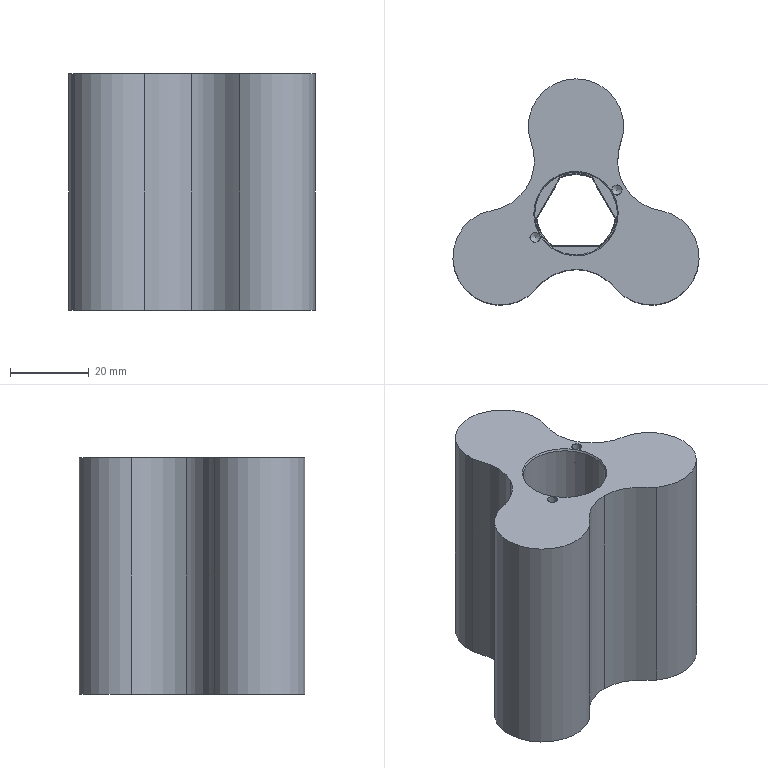NC program | NX | posted with a generic post | part box 62.563 x 57.43 x 60 mm
Lines 7512 to 7567 of 9902:
(PLANAR_MILL_COPY_COPY_COPY , TOOL : D6A45)
N15022 T07 M6
N15024 G54
N15026 G17 G0 G90 X-21.777 Y2.353 S7500 M3
N15028 G43 Z30. H7
N15030 Z1.5
N15032 G94 G1 Z-1.5 F1250.
N15034 G3 X-20.946 Y2.202 R1.
N15036 X-19.459 Y2.664 R17.938
N15038 X-17.28 Y3.717 R11.484
N15040 X-15.09 Y5.484 R11.427
N15042 X-13.385 Y7.728 R11.903
N15044 X-12.293 Y10.328 R11.906
N15046 X-11.858 Y13.109 R11.425
N15048 X-12.037 Y15.524 R11.478
N15050 X-12.66 Y17.967 R17.993
N15052 G2 X-13.077 Y19.319 R33.137
N15054 X-13.37 Y20.886 R8.649
N15056 X13.37 Y20.885 R-13.426
N15058 X13.233 Y19.945 R9.288
N15060 X13.008 Y19.033 R9.941
N15062 X12.741 Y18.203 R20.194
N15064 G3 X12.499 Y17.467 R24.527
N15066 X12.12 Y16.015 R16.385
N15068 X11.902 Y14.567 R12.285
N15070 X12.121 Y11.032 R11.667
N15072 X13.385 Y7.728 R11.771
N15074 X15.091 Y5.482 R11.906
N15076 X17.282 Y3.715 R11.425
N15078 X19.463 Y2.663 R11.478
N15080 X21.89 Y1.981 R17.993
N15082 G2 X23.269 Y1.665 R33.137
N15084 X24.773 Y1.135 R8.649
N15086 X11.402 Y-22.021 R-13.426
N15088 X10.19 Y-20.982 R8.649
N15090 X9.226 Y-19.943 R33.605
N15092 G3 X7.422 Y-18.184 R17.938
N15094 X5.421 Y-16.823 R11.484
N15096 X2.796 Y-15.81 R11.427
N15098 X0. Y-15.455 R11.903
N15100 X-2.798 Y-15.81 R11.906
N15102 X-5.424 Y-16.824 R11.425
N15104 X-7.425 Y-18.186 R11.478
N15106 X-9.23 Y-19.948 R17.993
N15108 G2 X-10.193 Y-20.984 R33.137
N15110 X-11.403 Y-22.022 R8.649
N15112 X-24.772 Y1.136 R-13.426
N15114 X-23.266 Y1.666 R8.649
N15116 X-21.884 Y1.982 R33.605
N15118 G3 X-20.946 Y2.202 R17.938
N15120 X-20.296 Y2.743 R1.
N15122 G1 Z1.5
N15124 G0 Z30.
N15126 M5